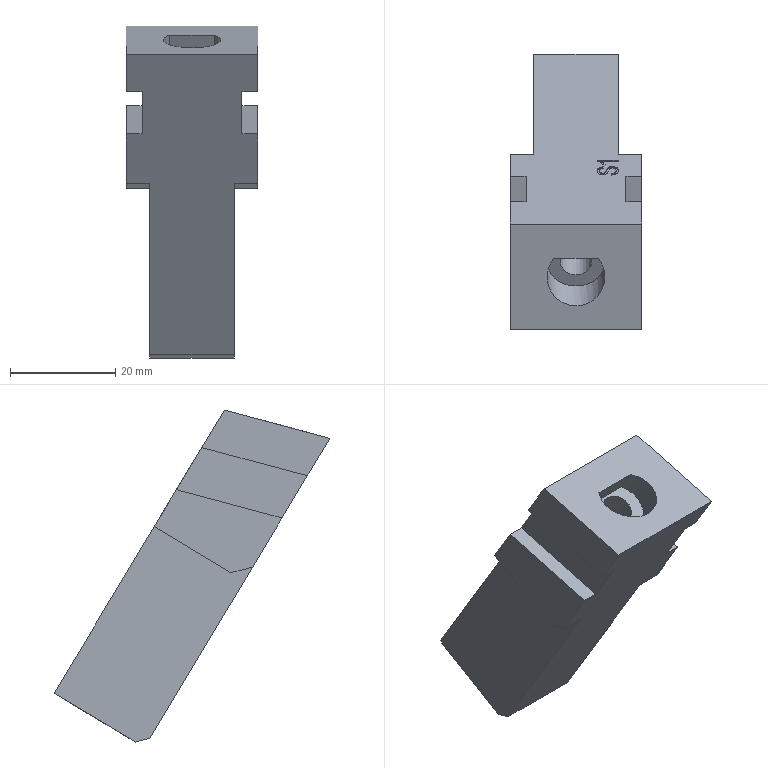Part | STEP file | lll_id34_x_t | 1 solid | 55 faces | box 25 x 52.484 x 63.172 mm | volume 22828 mm3 | plane 32 | other 21 | cylinder 2 | commonest cylinder face diameters 6 x1 11 x1